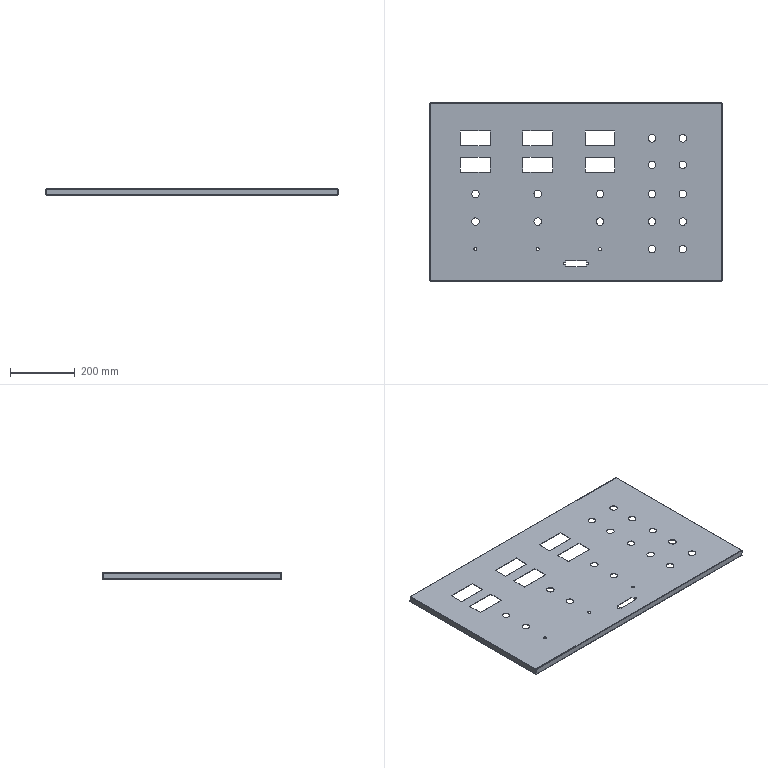Part | SolidWorks | features EdgeFlange 2, ICE 2, FlatPattern 1, SMBaseFlange 1, SheetMetal 1 | 1 solid | 145 faces | box 900 x 550 x 20 mm | volume 805688 mm3 | plane 72 | cylinder 57 | spline 16 | commonest cylinder face diameters 23 x32 0.2 x8 3.2 x8 9 x6 7 x3